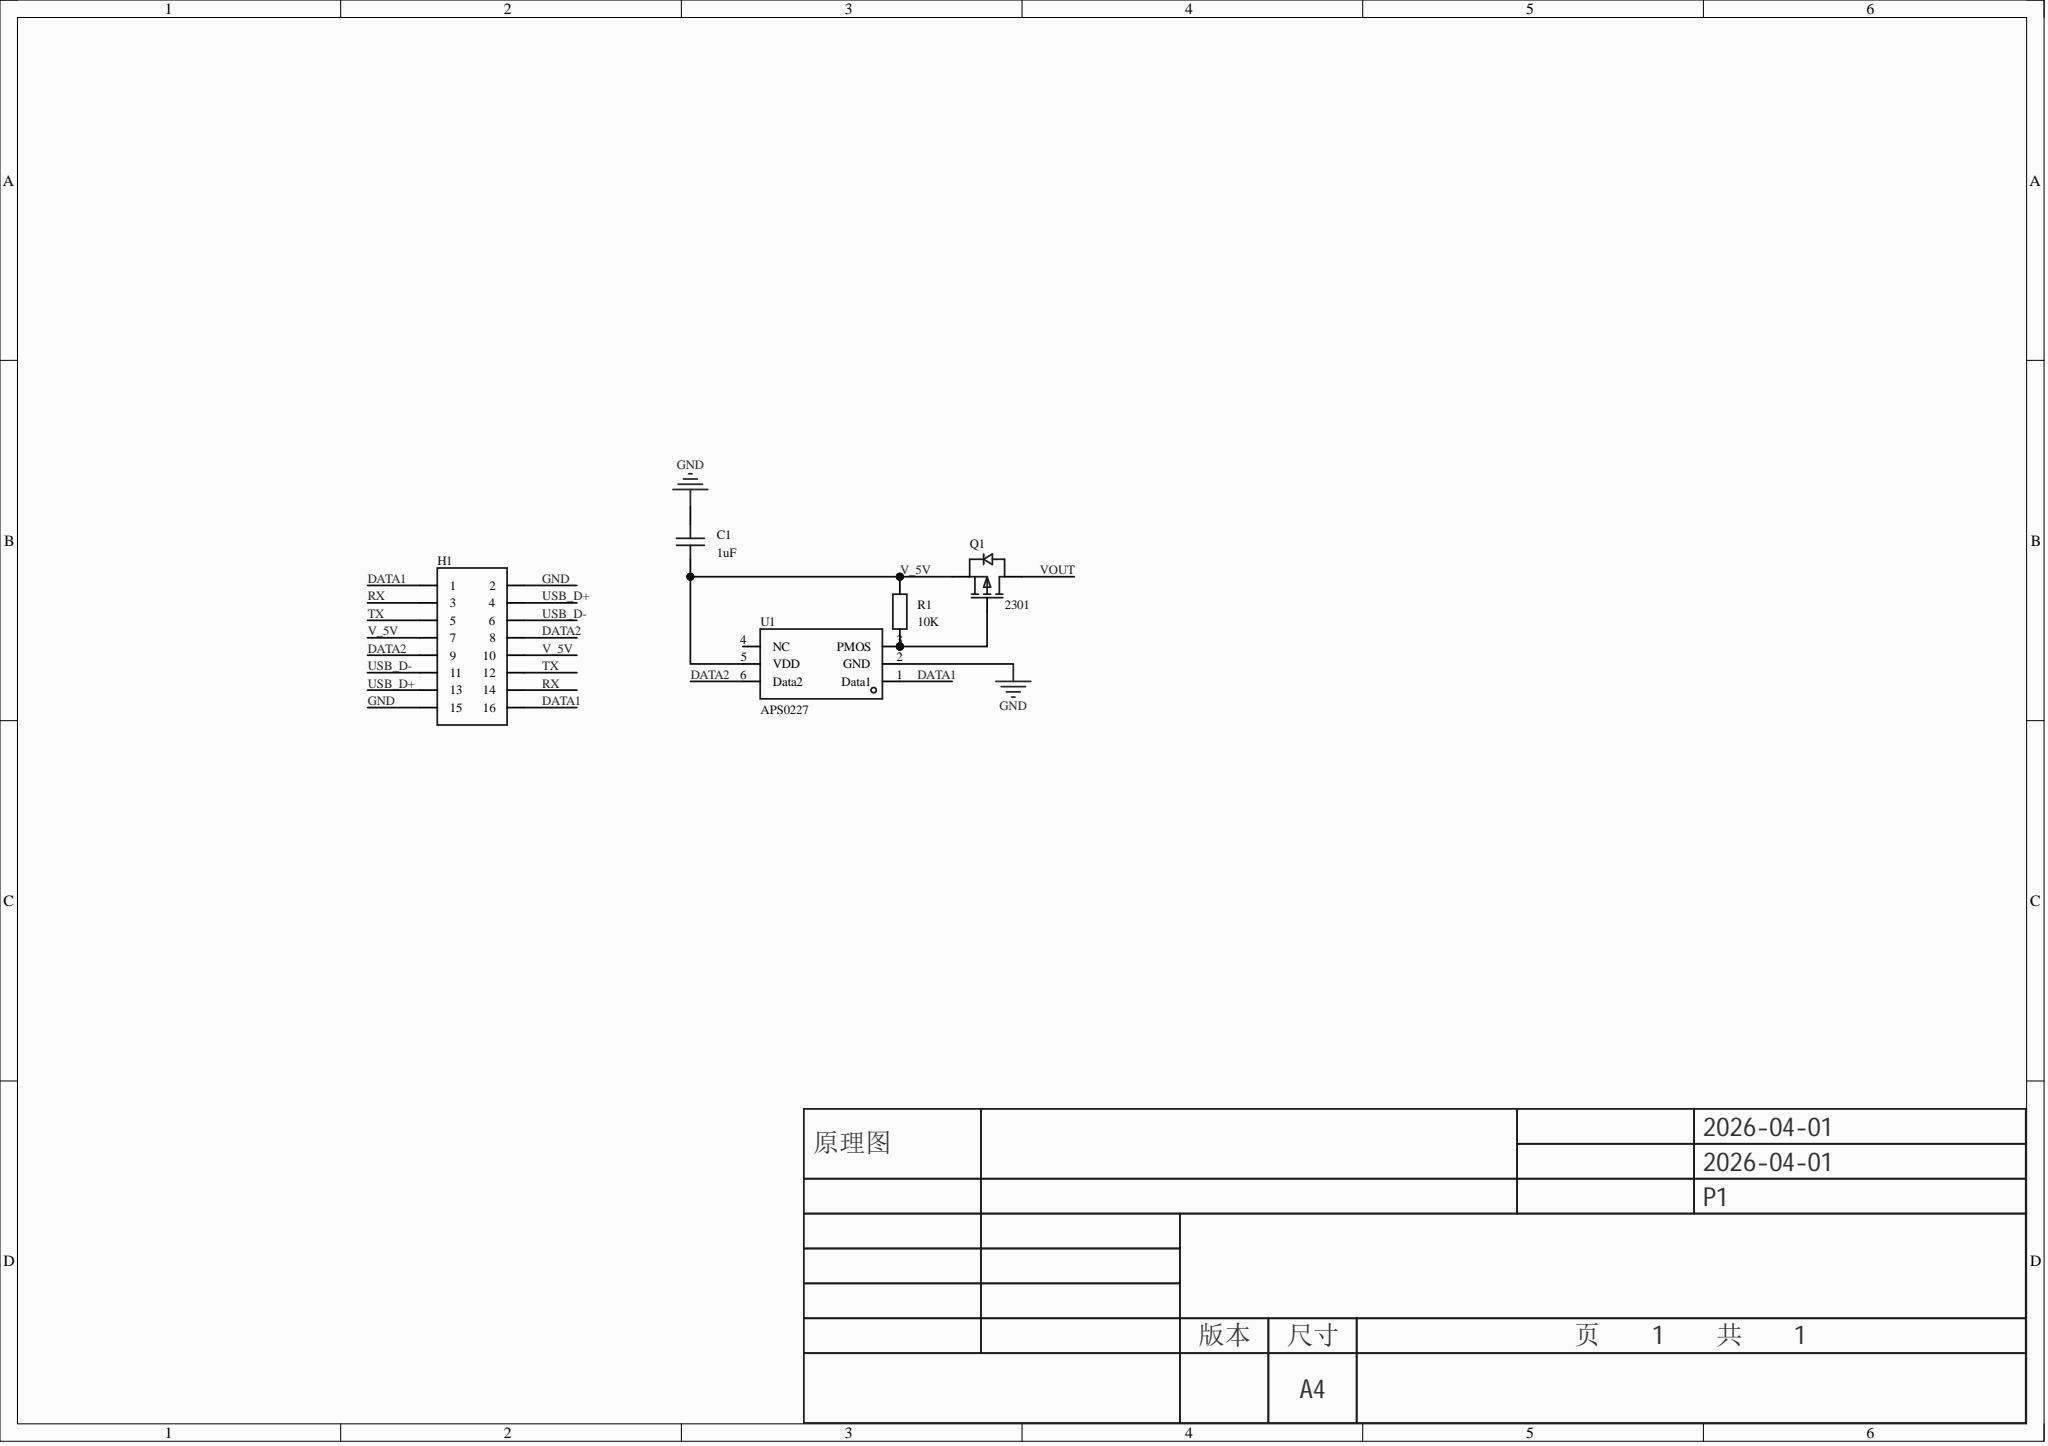Circuit board | Altium Designer | 5 parts | 9 nets
Bill of materials:
Comment,Description,Designator,Footprint,LibRef,Quantity
"1uF","","C1","C0402","CAP_0402","1"
"","","H1","HDR-TH_16P-P2.54-V-F-R2-C8-S2.54-1","HDR-F_2.54_2x8","1"
"2301","","Q1","SOT-23-3_L3.0-W1.7-P0.95-LS2.9-BR","SI2301CDS-T1-GE3","1"
"10K","","R1","R0402","Res_0402","1"
"APS0227","","U1","TSOT-23-6_L2.9-W1.6-P0.95-LS2.8-BR","APS0227","1"
Netlist (Protel format):
[
C1
C0402
1uF



]
[
H1
HDR-TH_16P-P2.54-V-F-R2-C8-S2.54-1




]
[
Q1
SOT-23-3_L3.0-W1.7-P0.95-LS2.9-BR
2301



]
[
R1
R0402
10K



]
[
U1
TSOT-23-6_L2.9-W1.6-P0.95-LS2.8-BR
APS0227



]
(
V_5V
C1-1
H1-7
H1-10
Q1-2
R1-2
U1-5
)
(
USB_D-
H1-6
H1-11
)
(
USB_D+
H1-4
H1-13
)
(
TX
H1-5
H1-12
)
(
RX
H1-3
H1-14
)
(
NetQ1_1
Q1-1
R1-1
U1-3
)
(
GND
C1-2
H1-2
H1-15
U1-2
)
(
DATA2
H1-8
H1-9
U1-6
)
(
DATA1
H1-1
H1-16
U1-1
)